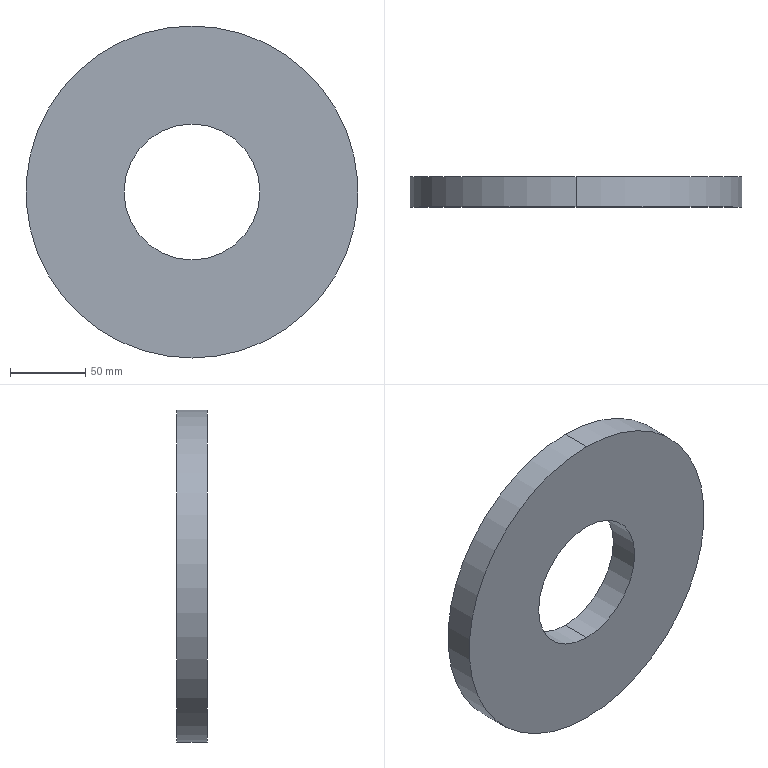Part | SolidWorks | features Extrusion 1 | 1 solid | 6 faces | box 220 x 20 x 220 mm | volume 633031 mm3 | cylinder 4 | plane 2 | commonest cylinder face diameters 90 x2 220 x2
STEP:
#1=CARTESIAN_POINT('',(0.,20.,-45.));
#2=VERTEX_POINT('',#1);
#3=CARTESIAN_POINT('',(0.,20.,45.));
#4=VERTEX_POINT('',#3);
#5=CARTESIAN_POINT('',(0.,20.,0.));
#6=DIRECTION('',(0.,1.,0.));
#7=DIRECTION('',(0.,0.,1.));
#8=AXIS2_PLACEMENT_3D('',#5,#6,#7);
#9=CIRCLE('',#8,45.);
#10=EDGE_CURVE('',#2,#4,#9,.T.);
#11=ORIENTED_EDGE('',*,*,#10,.T.);
#12=CARTESIAN_POINT('',(0.,0.,45.));
#13=VERTEX_POINT('',#12);
#14=CARTESIAN_POINT('',(0.,20.,45.));
#15=DIRECTION('',(0.,-1.,0.));
#16=VECTOR('',#15,1000.);
#17=LINE('',#14,#16);
#18=EDGE_CURVE('',#4,#13,#17,.T.);
#19=ORIENTED_EDGE('',*,*,#18,.T.);
#20=CARTESIAN_POINT('',(0.,0.,-45.));
#21=VERTEX_POINT('',#20);
#22=CARTESIAN_POINT('',(0.,0.,0.));
#23=DIRECTION('',(0.,1.,0.));
#24=DIRECTION('',(0.,0.,1.));
#25=AXIS2_PLACEMENT_3D('',#22,#23,#24);
#26=CIRCLE('',#25,45.);
#27=EDGE_CURVE('',#21,#13,#26,.T.);
#28=ORIENTED_EDGE('',*,*,#27,.F.);
#29=CARTESIAN_POINT('',(0.,20.,-45.));
#30=DIRECTION('',(0.,-1.,0.));
#31=VECTOR('',#30,1000.);
#32=LINE('',#29,#31);
#33=EDGE_CURVE('',#2,#21,#32,.T.);
#34=ORIENTED_EDGE('',*,*,#33,.F.);
#35=EDGE_LOOP('',(#11,#19,#28,#34));
#36=FACE_OUTER_BOUND('',#35,.T.);
#37=CARTESIAN_POINT('',(0.,20.,0.));
#38=DIRECTION('',(0.,-1.,0.));
#39=DIRECTION('',(0.,0.,-1.));
#40=AXIS2_PLACEMENT_3D('',#37,#38,#39);
#41=CYLINDRICAL_SURFACE('',#40,45.);
#42=ADVANCED_FACE('',(#36),#41,.F.);
#43=CARTESIAN_POINT('',(0.,20.,110.));
#44=VERTEX_POINT('',#43);
#45=CARTESIAN_POINT('',(0.,20.,-110.));
#46=VERTEX_POINT('',#45);
#47=CARTESIAN_POINT('',(0.,20.,0.));
#48=DIRECTION('',(0.,1.,0.));
#49=DIRECTION('',(0.,0.,1.));
#50=AXIS2_PLACEMENT_3D('',#47,#48,#49);
#51=CIRCLE('',#50,110.);
#52=EDGE_CURVE('',#44,#46,#51,.T.);
#53=ORIENTED_EDGE('',*,*,#52,.F.);
#54=CARTESIAN_POINT('',(0.,0.,110.));
#55=VERTEX_POINT('',#54);
#56=CARTESIAN_POINT('',(0.,20.,110.));
#57=DIRECTION('',(0.,-1.,0.));
#58=VECTOR('',#57,1000.);
#59=LINE('',#56,#58);
#60=EDGE_CURVE('',#44,#55,#59,.T.);
#61=ORIENTED_EDGE('',*,*,#60,.T.);
#62=CARTESIAN_POINT('',(0.,0.,-110.));
#63=VERTEX_POINT('',#62);
#64=CARTESIAN_POINT('',(0.,0.,0.));
#65=DIRECTION('',(0.,1.,0.));
#66=DIRECTION('',(0.,0.,1.));
#67=AXIS2_PLACEMENT_3D('',#64,#65,#66);
#68=CIRCLE('',#67,110.);
#69=EDGE_CURVE('',#55,#63,#68,.T.);
#70=ORIENTED_EDGE('',*,*,#69,.T.);
#71=CARTESIAN_POINT('',(0.,20.,-110.));
#72=DIRECTION('',(0.,-1.,0.));
#73=VECTOR('',#72,1000.);
#74=LINE('',#71,#73);
#75=EDGE_CURVE('',#46,#63,#74,.T.);
#76=ORIENTED_EDGE('',*,*,#75,.F.);
#77=EDGE_LOOP('',(#53,#61,#70,#76));
#78=FACE_OUTER_BOUND('',#77,.T.);
#79=CARTESIAN_POINT('',(0.,20.,0.));
#80=DIRECTION('',(0.,-1.,0.));
#81=DIRECTION('',(0.,0.,-1.));
#82=AXIS2_PLACEMENT_3D('',#79,#80,#81);
#83=CYLINDRICAL_SURFACE('',#82,110.);
#84=ADVANCED_FACE('',(#78),#83,.T.);
#85=CARTESIAN_POINT('',(0.,20.,0.));
#86=DIRECTION('',(0.,1.,0.));
#87=DIRECTION('',(0.,0.,1.));
#88=AXIS2_PLACEMENT_3D('',#85,#86,#87);
#89=CIRCLE('',#88,110.);
#90=EDGE_CURVE('',#46,#44,#89,.T.);
#91=ORIENTED_EDGE('',*,*,#90,.T.);
#92=ORIENTED_EDGE('',*,*,#52,.T.);
#93=EDGE_LOOP('',(#91,#92));
#94=FACE_OUTER_BOUND('',#93,.T.);
#95=ORIENTED_EDGE('',*,*,#10,.F.);
#96=CARTESIAN_POINT('',(0.,20.,0.));
#97=DIRECTION('',(0.,1.,0.));
#98=DIRECTION('',(0.,0.,1.));
#99=AXIS2_PLACEMENT_3D('',#96,#97,#98);
#100=CIRCLE('',#99,45.);
#101=EDGE_CURVE('',#4,#2,#100,.T.);
#102=ORIENTED_EDGE('',*,*,#101,.F.);
#103=EDGE_LOOP('',(#95,#102));
#104=FACE_BOUND('',#103,.T.);
#105=CARTESIAN_POINT('',(0.,20.,0.));
#106=DIRECTION('',(0.,1.,0.));
#107=DIRECTION('',(0.,0.,1.));
#108=AXIS2_PLACEMENT_3D('',#105,#106,#107);
#109=PLANE('',#108);
#110=ADVANCED_FACE('',(#94,#104),#109,.T.);
#111=CARTESIAN_POINT('',(0.,0.,0.));
#112=DIRECTION('',(0.,1.,0.));
#113=DIRECTION('',(0.,0.,1.));
#114=AXIS2_PLACEMENT_3D('',#111,#112,#113);
#115=CIRCLE('',#114,110.);
#116=EDGE_CURVE('',#63,#55,#115,.T.);
#117=ORIENTED_EDGE('',*,*,#116,.F.);
#118=ORIENTED_EDGE('',*,*,#69,.F.);
#119=EDGE_LOOP('',(#117,#118));
#120=FACE_OUTER_BOUND('',#119,.T.);
#121=ORIENTED_EDGE('',*,*,#27,.T.);
#122=CARTESIAN_POINT('',(0.,0.,0.));
#123=DIRECTION('',(0.,1.,0.));
#124=DIRECTION('',(0.,0.,1.));
#125=AXIS2_PLACEMENT_3D('',#122,#123,#124);
#126=CIRCLE('',#125,45.);
#127=EDGE_CURVE('',#13,#21,#126,.T.);
#128=ORIENTED_EDGE('',*,*,#127,.T.);
#129=EDGE_LOOP('',(#121,#128));
#130=FACE_BOUND('',#129,.T.);
#131=CARTESIAN_POINT('',(0.,0.,0.));
#132=DIRECTION('',(0.,1.,0.));
#133=DIRECTION('',(0.,0.,1.));
#134=AXIS2_PLACEMENT_3D('',#131,#132,#133);
#135=PLANE('',#134);
#136=ADVANCED_FACE('',(#120,#130),#135,.F.);
#137=ORIENTED_EDGE('',*,*,#60,.F.);
#138=ORIENTED_EDGE('',*,*,#90,.F.);
#139=ORIENTED_EDGE('',*,*,#75,.T.);
#140=ORIENTED_EDGE('',*,*,#116,.T.);
#141=EDGE_LOOP('',(#137,#138,#139,#140));
#142=FACE_OUTER_BOUND('',#141,.T.);
#143=CARTESIAN_POINT('',(0.,20.,0.));
#144=DIRECTION('',(0.,-1.,0.));
#145=DIRECTION('',(0.,0.,-1.));
#146=AXIS2_PLACEMENT_3D('',#143,#144,#145);
#147=CYLINDRICAL_SURFACE('',#146,110.);
#148=ADVANCED_FACE('',(#142),#147,.T.);
#149=ORIENTED_EDGE('',*,*,#18,.F.);
#150=ORIENTED_EDGE('',*,*,#101,.T.);
#151=ORIENTED_EDGE('',*,*,#33,.T.);
#152=ORIENTED_EDGE('',*,*,#127,.F.);
#153=EDGE_LOOP('',(#149,#150,#151,#152));
#154=FACE_OUTER_BOUND('',#153,.T.);
#155=CARTESIAN_POINT('',(0.,20.,0.));
#156=DIRECTION('',(0.,-1.,0.));
#157=DIRECTION('',(0.,0.,-1.));
#158=AXIS2_PLACEMENT_3D('',#155,#156,#157);
#159=CYLINDRICAL_SURFACE('',#158,45.);
#160=ADVANCED_FACE('',(#154),#159,.F.);
#161=CLOSED_SHELL('',(#42,#84,#110,#136,#148,#160));
#162=MANIFOLD_SOLID_BREP('',#161);
#163=CARTESIAN_POINT('',(0.,0.,0.));
#164=DIRECTION('',(0.,0.,1.));
#165=DIRECTION('',(1.,0.,0.));
#166=AXIS2_PLACEMENT_3D('',#163,#164,#165);
#167=(LENGTH_UNIT()NAMED_UNIT(*)SI_UNIT(.MILLI.,.METRE.));
#168=UNCERTAINTY_MEASURE_WITH_UNIT(LENGTH_MEASURE(0.00001),#167,'','');
#169=(NAMED_UNIT(*)PLANE_ANGLE_UNIT()SI_UNIT($,.RADIAN.));
#170=(NAMED_UNIT(*)SI_UNIT($,.STERADIAN.)SOLID_ANGLE_UNIT());
#171=(GEOMETRIC_REPRESENTATION_CONTEXT(3)GLOBAL_UNCERTAINTY_ASSIGNED_CONTEXT((#168))GLOBAL_UNIT_ASSIGNED_CONTEXT((#167,#169,#170))REPRESENTATION_CONTEXT('',''));
#172=ADVANCED_BREP_SHAPE_REPRESENTATION('',(#162,#166),#171);